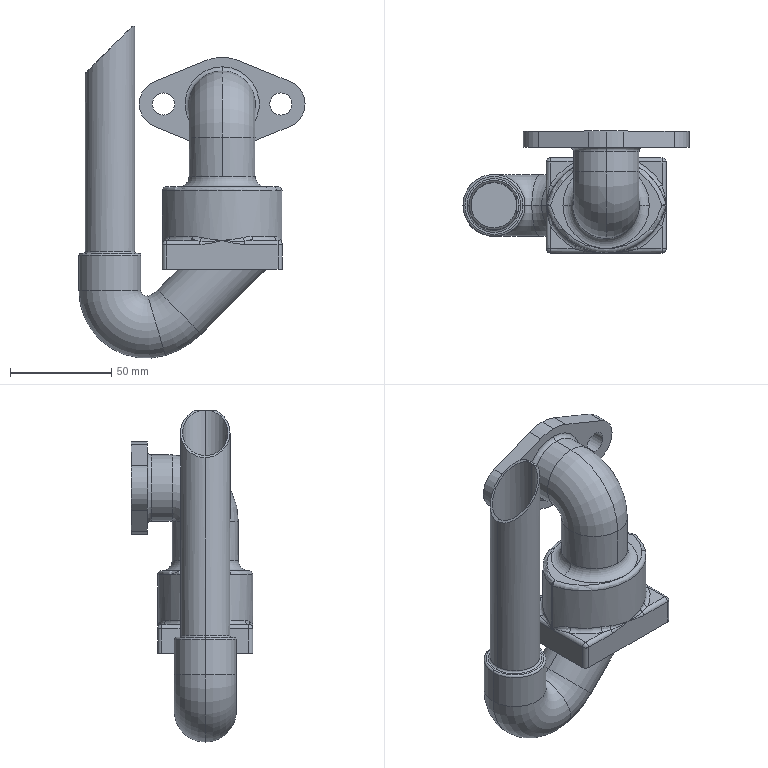Part | SolidWorks | features BaseBody 1 | 1 solid | 117 faces | box 111.824 x 60.133 x 164.223 mm | volume 200777 mm3 | cylinder 43 | torus 26 | plane 23 | spline 18 | sphere 7 | commonest cylinder face diameters 4.089 x12 22.489 x6 11 x4 16.356 x4 30.667 x4 32.711 x4